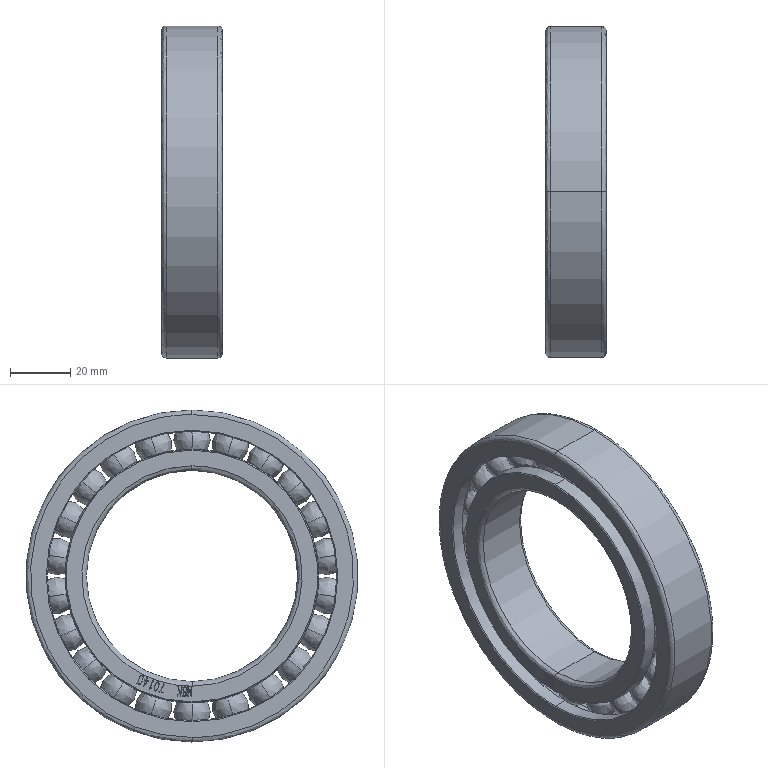Part | STEP file | 7014C | 1 solid | 304 faces | box 20 x 110 x 110 mm | volume 86450 mm3 | spline 180 | plane 104 | cylinder 12 | cone 8 | commonest cylinder face diameters 84 x4 96 x4 70 x2 110 x2